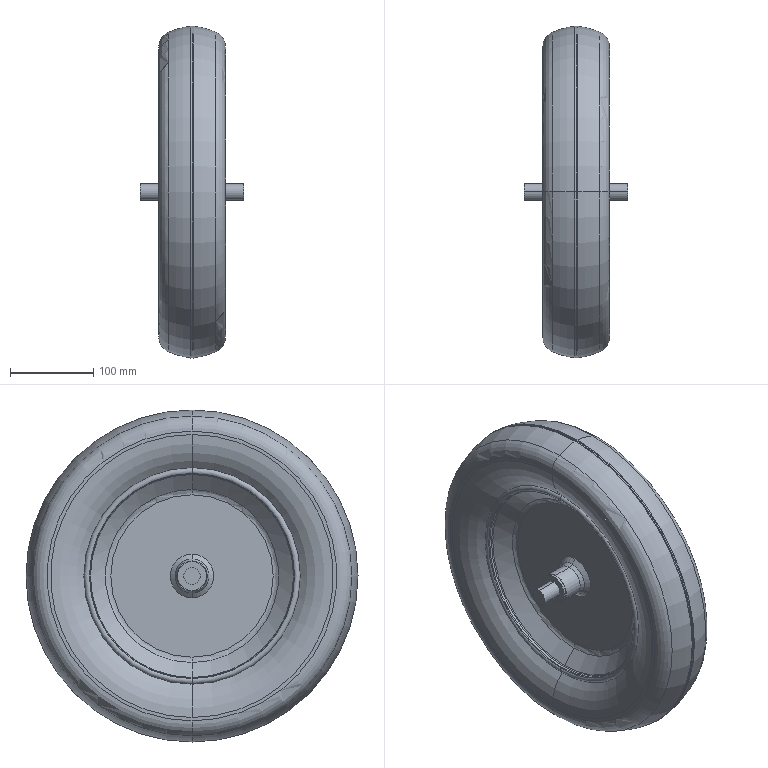Part | SolidWorks | features Revolution 2, ICE 1, MirrorSolid 1 | 2 solids | 164 faces | box 125 x 399.062 x 399.062 mm | volume 898326 mm3 | torus 72 | cylinder 38 | cone 36 | plane 18 | commonest cylinder face diameters 20 x6 33.4 x4 35 x4 36.4 x4 245.5 x4 248.5 x4